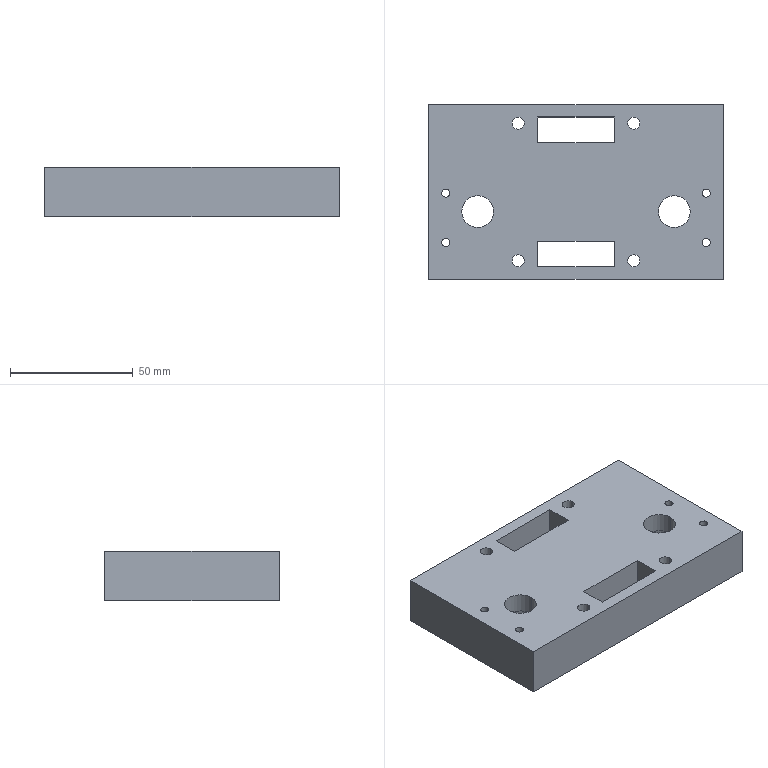Part | 1 solid | 75 faces | box 120 x 71 x 20 mm | volume 135638 mm3 | cylinder 40 | plane 19 | cone 16 | commonest cylinder face diameters 3.3 x24 5 x8 13 x4 19 x4